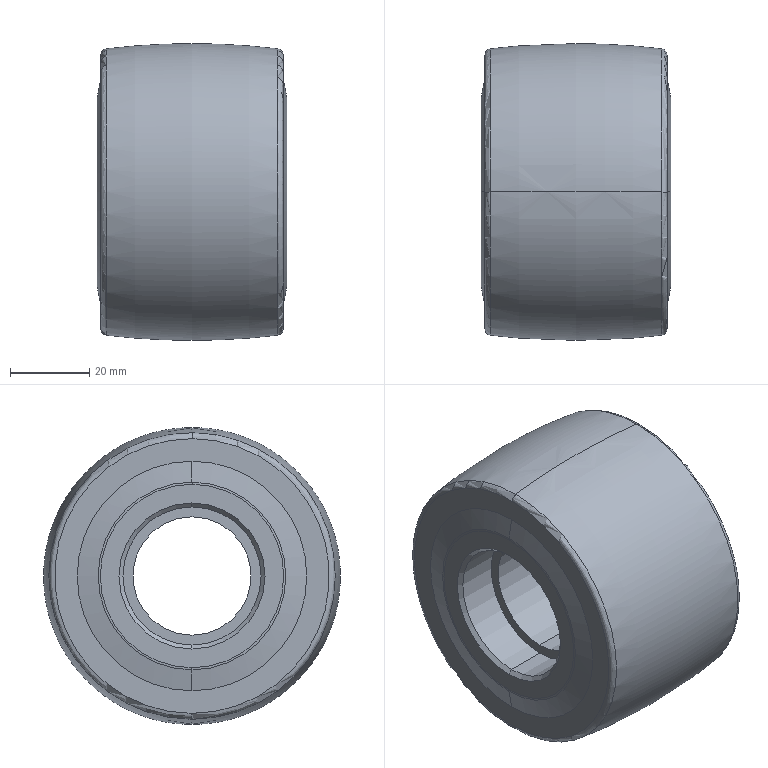Part | NX | features solid 2 | 1 solid | 30 faces | box 48 x 75 x 75 mm | volume 162673 mm3 | torus 10 | cone 8 | cylinder 6 | plane 6 | commonest cylinder face diameters 34.9 x4 29.9 x2
STEP:
#1=CARTESIAN_POINT('',(177.1,-71.5,-939.05));
#2=VERTEX_POINT('',#1);
#3=CARTESIAN_POINT('',(202.9,-71.5,-939.05));
#4=VERTEX_POINT('',#3);
#5=CARTESIAN_POINT('',(202.9,-71.5,-939.05));
#6=DIRECTION('',(-1.,0.,0.));
#7=VECTOR('',#6,1000.);
#8=LINE('',#5,#7);
#9=EDGE_CURVE('',#2,#4,#8,.F.);
#10=ORIENTED_EDGE('',*,*,#9,.T.);
#11=CARTESIAN_POINT('',(202.9,-71.5,-968.95));
#12=VERTEX_POINT('',#11);
#13=CARTESIAN_POINT('',(202.9,-71.5,-954.));
#14=DIRECTION('',(1.,0.,0.));
#15=DIRECTION('',(0.,0.,1.));
#16=AXIS2_PLACEMENT_3D('',#13,#14,#15);
#17=CIRCLE('',#16,14.95);
#18=EDGE_CURVE('',#4,#12,#17,.T.);
#19=ORIENTED_EDGE('',*,*,#18,.T.);
#20=CARTESIAN_POINT('',(177.1,-71.5,-968.95));
#21=VERTEX_POINT('',#20);
#22=CARTESIAN_POINT('',(202.9,-71.5,-968.95));
#23=DIRECTION('',(-1.,0.,0.));
#24=VECTOR('',#23,1000.);
#25=LINE('',#22,#24);
#26=EDGE_CURVE('',#12,#21,#25,.T.);
#27=ORIENTED_EDGE('',*,*,#26,.T.);
#28=CARTESIAN_POINT('',(177.1,-71.5,-954.));
#29=DIRECTION('',(-1.,0.,0.));
#30=DIRECTION('',(0.,0.,-1.));
#31=AXIS2_PLACEMENT_3D('',#28,#29,#30);
#32=CIRCLE('',#31,14.95);
#33=EDGE_CURVE('',#21,#2,#32,.T.);
#34=ORIENTED_EDGE('',*,*,#33,.T.);
#35=EDGE_LOOP('',(#10,#19,#27,#34));
#36=FACE_BOUND('',#35,.T.);
#37=CARTESIAN_POINT('',(163.6,-71.5,-954.));
#38=DIRECTION('',(1.,0.,0.));
#39=DIRECTION('',(0.,0.,1.));
#40=AXIS2_PLACEMENT_3D('',#37,#38,#39);
#41=CYLINDRICAL_SURFACE('',#40,14.95);
#42=ADVANCED_FACE('',(#36),#41,.F.);
#43=CARTESIAN_POINT('',(177.1,-71.5,-971.45));
#44=VERTEX_POINT('',#43);
#45=CARTESIAN_POINT('',(177.1,-71.5,-936.55));
#46=VERTEX_POINT('',#45);
#47=CARTESIAN_POINT('',(177.1,-71.5,-954.));
#48=DIRECTION('',(1.,0.,0.));
#49=DIRECTION('',(0.,0.,-1.));
#50=AXIS2_PLACEMENT_3D('',#47,#48,#49);
#51=CIRCLE('',#50,17.45);
#52=EDGE_CURVE('',#44,#46,#51,.T.);
#53=ORIENTED_EDGE('',*,*,#52,.F.);
#54=CARTESIAN_POINT('',(177.1,-71.5,-954.));
#55=DIRECTION('',(1.,0.,0.));
#56=DIRECTION('',(0.,0.,1.));
#57=AXIS2_PLACEMENT_3D('',#54,#55,#56);
#58=CIRCLE('',#57,17.45);
#59=EDGE_CURVE('',#46,#44,#58,.T.);
#60=ORIENTED_EDGE('',*,*,#59,.F.);
#61=EDGE_LOOP('',(#53,#60));
#62=FACE_BOUND('',#61,.T.);
#63=CARTESIAN_POINT('',(177.1,-71.5,-954.));
#64=DIRECTION('',(-1.,0.,0.));
#65=DIRECTION('',(0.,0.,1.));
#66=AXIS2_PLACEMENT_3D('',#63,#64,#65);
#67=CIRCLE('',#66,14.95);
#68=EDGE_CURVE('',#2,#21,#67,.T.);
#69=ORIENTED_EDGE('',*,*,#68,.F.);
#70=ORIENTED_EDGE('',*,*,#33,.F.);
#71=EDGE_LOOP('',(#69,#70));
#72=FACE_BOUND('',#71,.T.);
#73=CARTESIAN_POINT('',(177.1,-71.5,-954.));
#74=DIRECTION('',(1.,0.,0.));
#75=DIRECTION('',(0.,0.,1.));
#76=AXIS2_PLACEMENT_3D('',#73,#74,#75);
#77=PLANE('',#76);
#78=ADVANCED_FACE('',(#62,#72),#77,.F.);
#79=CARTESIAN_POINT('',(167.,-71.5,-936.55));
#80=VERTEX_POINT('',#79);
#81=CARTESIAN_POINT('',(177.1,-71.5,-936.55));
#82=DIRECTION('',(-1.,0.,0.));
#83=VECTOR('',#82,1000.);
#84=LINE('',#81,#83);
#85=EDGE_CURVE('',#80,#46,#84,.F.);
#86=ORIENTED_EDGE('',*,*,#85,.T.);
#87=ORIENTED_EDGE('',*,*,#59,.T.);
#88=CARTESIAN_POINT('',(167.,-71.5,-971.45));
#89=VERTEX_POINT('',#88);
#90=CARTESIAN_POINT('',(177.1,-71.5,-971.45));
#91=DIRECTION('',(-1.,0.,0.));
#92=VECTOR('',#91,1000.);
#93=LINE('',#90,#92);
#94=EDGE_CURVE('',#44,#89,#93,.T.);
#95=ORIENTED_EDGE('',*,*,#94,.T.);
#96=CARTESIAN_POINT('',(167.,-71.5,-954.));
#97=DIRECTION('',(-1.,0.,0.));
#98=DIRECTION('',(0.,0.,-1.));
#99=AXIS2_PLACEMENT_3D('',#96,#97,#98);
#100=CIRCLE('',#99,17.45);
#101=EDGE_CURVE('',#89,#80,#100,.T.);
#102=ORIENTED_EDGE('',*,*,#101,.T.);
#103=EDGE_LOOP('',(#86,#87,#95,#102));
#104=FACE_BOUND('',#103,.T.);
#105=CARTESIAN_POINT('',(163.6,-71.5,-954.));
#106=DIRECTION('',(1.,0.,0.));
#107=DIRECTION('',(0.,0.,1.));
#108=AXIS2_PLACEMENT_3D('',#105,#106,#107);
#109=CYLINDRICAL_SURFACE('',#108,17.45);
#110=ADVANCED_FACE('',(#104),#109,.F.);
#111=CARTESIAN_POINT('',(166.,-71.5,-972.45));
#112=VERTEX_POINT('',#111);
#113=CARTESIAN_POINT('',(166.,-71.5,-972.45));
#114=DIRECTION('',(0.7071,0.,0.7071));
#115=VECTOR('',#114,1000.);
#116=LINE('',#113,#115);
#117=EDGE_CURVE('',#112,#89,#116,.T.);
#118=ORIENTED_EDGE('',*,*,#117,.F.);
#119=CARTESIAN_POINT('',(166.,-71.5,-935.55));
#120=VERTEX_POINT('',#119);
#121=CARTESIAN_POINT('',(166.,-71.5,-954.));
#122=DIRECTION('',(-1.,0.,0.));
#123=DIRECTION('',(0.,0.,-1.));
#124=AXIS2_PLACEMENT_3D('',#121,#122,#123);
#125=CIRCLE('',#124,18.45);
#126=EDGE_CURVE('',#112,#120,#125,.T.);
#127=ORIENTED_EDGE('',*,*,#126,.T.);
#128=CARTESIAN_POINT('',(166.,-71.5,-935.55));
#129=DIRECTION('',(0.7071,0.,-0.7071));
#130=VECTOR('',#129,1000.);
#131=LINE('',#128,#130);
#132=EDGE_CURVE('',#80,#120,#131,.F.);
#133=ORIENTED_EDGE('',*,*,#132,.F.);
#134=ORIENTED_EDGE('',*,*,#101,.F.);
#135=EDGE_LOOP('',(#118,#127,#133,#134));
#136=FACE_BOUND('',#135,.T.);
#137=CARTESIAN_POINT('',(166.5,-71.5,-954.));
#138=DIRECTION('',(-1.,0.,0.));
#139=DIRECTION('',(0.,0.,-1.));
#140=AXIS2_PLACEMENT_3D('',#137,#138,#139);
#141=CONICAL_SURFACE('',#140,17.95,0.7854);
#142=ADVANCED_FACE('',(#136),#141,.F.);
#143=CARTESIAN_POINT('',(167.,-71.5,-954.));
#144=DIRECTION('',(-1.,0.,0.));
#145=DIRECTION('',(0.,0.,1.));
#146=AXIS2_PLACEMENT_3D('',#143,#144,#145);
#147=CIRCLE('',#146,17.45);
#148=EDGE_CURVE('',#80,#89,#147,.T.);
#149=ORIENTED_EDGE('',*,*,#148,.F.);
#150=ORIENTED_EDGE('',*,*,#132,.T.);
#151=CARTESIAN_POINT('',(166.,-71.5,-954.));
#152=DIRECTION('',(-1.,0.,0.));
#153=DIRECTION('',(0.,0.,1.));
#154=AXIS2_PLACEMENT_3D('',#151,#152,#153);
#155=CIRCLE('',#154,18.45);
#156=EDGE_CURVE('',#120,#112,#155,.T.);
#157=ORIENTED_EDGE('',*,*,#156,.T.);
#158=ORIENTED_EDGE('',*,*,#117,.T.);
#159=EDGE_LOOP('',(#149,#150,#157,#158));
#160=FACE_BOUND('',#159,.T.);
#161=CARTESIAN_POINT('',(166.5,-71.5,-954.));
#162=DIRECTION('',(-1.,0.,0.));
#163=DIRECTION('',(0.,0.,-1.));
#164=AXIS2_PLACEMENT_3D('',#161,#162,#163);
#165=CONICAL_SURFACE('',#164,17.95,0.7854);
#166=ADVANCED_FACE('',(#160),#165,.F.);
#167=CARTESIAN_POINT('',(166.,-71.724,-930.819));
#168=VERTEX_POINT('',#167);
#169=CARTESIAN_POINT('',(166.,-71.501,-977.182));
#170=VERTEX_POINT('',#169);
#171=CARTESIAN_POINT('',(166.,-71.5,-954.));
#172=DIRECTION('',(1.,0.,0.));
#173=DIRECTION('',(0.,-0.009654,1.));
#174=AXIS2_PLACEMENT_3D('',#171,#172,#173);
#175=CIRCLE('',#174,23.182);
#176=EDGE_CURVE('',#168,#170,#175,.T.);
#177=ORIENTED_EDGE('',*,*,#176,.F.);
#178=CARTESIAN_POINT('',(166.,-71.499,-930.818));
#179=VERTEX_POINT('',#178);
#180=CARTESIAN_POINT('',(166.,-71.5,-954.));
#181=DIRECTION('',(-1.,0.,0.));
#182=DIRECTION('',(0.,-0.009654,1.));
#183=AXIS2_PLACEMENT_3D('',#180,#181,#182);
#184=CIRCLE('',#183,23.182);
#185=EDGE_CURVE('',#168,#179,#184,.T.);
#186=ORIENTED_EDGE('',*,*,#185,.T.);
#187=CARTESIAN_POINT('',(166.,-71.276,-977.181));
#188=VERTEX_POINT('',#187);
#189=CARTESIAN_POINT('',(166.,-71.5,-954.));
#190=DIRECTION('',(1.,0.,0.));
#191=DIRECTION('',(0.,0.009654,-1.));
#192=AXIS2_PLACEMENT_3D('',#189,#190,#191);
#193=CIRCLE('',#192,23.182);
#194=EDGE_CURVE('',#179,#188,#193,.F.);
#195=ORIENTED_EDGE('',*,*,#194,.T.);
#196=CARTESIAN_POINT('',(166.,-71.5,-954.));
#197=DIRECTION('',(-1.,0.,0.));
#198=DIRECTION('',(0.,0.009654,-1.));
#199=AXIS2_PLACEMENT_3D('',#196,#197,#198);
#200=CIRCLE('',#199,23.182);
#201=EDGE_CURVE('',#170,#188,#200,.F.);
#202=ORIENTED_EDGE('',*,*,#201,.F.);
#203=EDGE_LOOP('',(#177,#186,#195,#202));
#204=FACE_BOUND('',#203,.T.);
#205=ORIENTED_EDGE('',*,*,#126,.F.);
#206=ORIENTED_EDGE('',*,*,#156,.F.);
#207=EDGE_LOOP('',(#205,#206));
#208=FACE_BOUND('',#207,.T.);
#209=CARTESIAN_POINT('',(166.,-71.5,-954.));
#210=DIRECTION('',(1.,0.,0.));
#211=DIRECTION('',(0.,0.,1.));
#212=AXIS2_PLACEMENT_3D('',#209,#210,#211);
#213=PLANE('',#212);
#214=ADVANCED_FACE('',(#204,#208),#213,.F.);
#215=CARTESIAN_POINT('',(166.048,-71.73,-930.287));
#216=VERTEX_POINT('',#215);
#217=CARTESIAN_POINT('',(169.,-71.725,-930.819));
#218=DIRECTION('',(0.,1.,0.009697));
#219=DIRECTION('',(-1.,0.000000003,-0.000000355));
#220=AXIS2_PLACEMENT_3D('',#217,#218,#219);
#221=CIRCLE('',#220,3.);
#222=EDGE_CURVE('',#168,#216,#221,.T.);
#223=ORIENTED_EDGE('',*,*,#222,.F.);
#224=ORIENTED_EDGE('',*,*,#176,.T.);
#225=ORIENTED_EDGE('',*,*,#201,.T.);
#226=CARTESIAN_POINT('',(166.048,-71.27,-977.713));
#227=VERTEX_POINT('',#226);
#228=CARTESIAN_POINT('',(169.,-71.275,-977.181));
#229=DIRECTION('',(0.,-1.,-0.009697));
#230=DIRECTION('',(-1.,-0.000000003,0.000000355));
#231=AXIS2_PLACEMENT_3D('',#228,#229,#230);
#232=CIRCLE('',#231,3.);
#233=EDGE_CURVE('',#227,#188,#232,.F.);
#234=ORIENTED_EDGE('',*,*,#233,.F.);
#235=CARTESIAN_POINT('',(166.048,-71.5,-977.714));
#236=VERTEX_POINT('',#235);
#237=CARTESIAN_POINT('',(166.048,-71.5,-954.));
#238=DIRECTION('',(1.,0.,0.));
#239=DIRECTION('',(0.,0.,-1.));
#240=AXIS2_PLACEMENT_3D('',#237,#238,#239);
#241=CIRCLE('',#240,23.714);
#242=EDGE_CURVE('',#236,#227,#241,.T.);
#243=ORIENTED_EDGE('',*,*,#242,.F.);
#244=CARTESIAN_POINT('',(166.048,-71.5,-954.));
#245=DIRECTION('',(1.,0.,0.));
#246=DIRECTION('',(0.,-0.009697,1.));
#247=AXIS2_PLACEMENT_3D('',#244,#245,#246);
#248=CIRCLE('',#247,23.714);
#249=EDGE_CURVE('',#216,#236,#248,.T.);
#250=ORIENTED_EDGE('',*,*,#249,.F.);
#251=EDGE_LOOP('',(#223,#224,#225,#234,#243,#250));
#252=FACE_BOUND('',#251,.T.);
#253=CARTESIAN_POINT('',(169.,-71.5,-954.));
#254=DIRECTION('',(-1.,0.,0.));
#255=DIRECTION('',(0.,0.009697,-1.));
#256=AXIS2_PLACEMENT_3D('',#253,#254,#255);
#257=TOROIDAL_SURFACE('',#256,23.182,3.);
#258=ADVANCED_FACE('',(#252),#257,.T.);
#259=CARTESIAN_POINT('',(166.048,-71.5,-930.286));
#260=VERTEX_POINT('',#259);
#261=CARTESIAN_POINT('',(166.048,-71.5,-954.));
#262=DIRECTION('',(1.,0.,0.));
#263=DIRECTION('',(0.,0.,1.));
#264=AXIS2_PLACEMENT_3D('',#261,#262,#263);
#265=CIRCLE('',#264,23.714);
#266=EDGE_CURVE('',#260,#216,#265,.T.);
#267=ORIENTED_EDGE('',*,*,#266,.T.);
#268=ORIENTED_EDGE('',*,*,#249,.T.);
#269=CARTESIAN_POINT('',(167.,-71.5,-983.));
#270=VERTEX_POINT('',#269);
#271=CARTESIAN_POINT('',(167.,-71.5,-983.));
#272=DIRECTION('',(-0.1773,0.,0.9842));
#273=VECTOR('',#272,1000.);
#274=LINE('',#271,#273);
#275=EDGE_CURVE('',#236,#270,#274,.F.);
#276=ORIENTED_EDGE('',*,*,#275,.T.);
#277=CARTESIAN_POINT('',(167.,-71.5,-925.));
#278=VERTEX_POINT('',#277);
#279=CARTESIAN_POINT('',(167.,-71.5,-954.));
#280=DIRECTION('',(-1.,0.,0.));
#281=DIRECTION('',(0.,0.,-1.));
#282=AXIS2_PLACEMENT_3D('',#279,#280,#281);
#283=CIRCLE('',#282,29.);
#284=EDGE_CURVE('',#270,#278,#283,.T.);
#285=ORIENTED_EDGE('',*,*,#284,.T.);
#286=CARTESIAN_POINT('',(167.,-71.5,-925.));
#287=DIRECTION('',(-0.1773,0.,-0.9842));
#288=VECTOR('',#287,1000.);
#289=LINE('',#286,#288);
#290=EDGE_CURVE('',#278,#260,#289,.T.);
#291=ORIENTED_EDGE('',*,*,#290,.T.);
#292=EDGE_LOOP('',(#267,#268,#276,#285,#291));
#293=FACE_BOUND('',#292,.T.);
#294=CARTESIAN_POINT('',(166.524,-71.5,-954.));
#295=DIRECTION('',(1.,0.,0.));
#296=DIRECTION('',(0.,0.,1.));
#297=AXIS2_PLACEMENT_3D('',#294,#295,#296);
#298=CONICAL_SURFACE('',#297,26.357,1.393);
#299=ADVANCED_FACE('',(#293),#298,.T.);
#300=CARTESIAN_POINT('',(166.048,-71.5,-954.));
#301=DIRECTION('',(1.,0.,0.));
#302=DIRECTION('',(0.,0.009697,-1.));
#303=AXIS2_PLACEMENT_3D('',#300,#301,#302);
#304=CIRCLE('',#303,23.714);
#305=EDGE_CURVE('',#227,#260,#304,.T.);
#306=ORIENTED_EDGE('',*,*,#305,.T.);
#307=ORIENTED_EDGE('',*,*,#290,.F.);
#308=CARTESIAN_POINT('',(167.,-71.5,-954.));
#309=DIRECTION('',(-1.,0.,0.));
#310=DIRECTION('',(0.,0.,1.));
#311=AXIS2_PLACEMENT_3D('',#308,#309,#310);
#312=CIRCLE('',#311,29.);
#313=EDGE_CURVE('',#278,#270,#312,.T.);
#314=ORIENTED_EDGE('',*,*,#313,.T.);
#315=ORIENTED_EDGE('',*,*,#275,.F.);
#316=ORIENTED_EDGE('',*,*,#242,.T.);
#317=EDGE_LOOP('',(#306,#307,#314,#315,#316));
#318=FACE_BOUND('',#317,.T.);
#319=CARTESIAN_POINT('',(166.524,-71.5,-954.));
#320=DIRECTION('',(1.,0.,0.));
#321=DIRECTION('',(0.,0.,1.));
#322=AXIS2_PLACEMENT_3D('',#319,#320,#321);
#323=CONICAL_SURFACE('',#322,26.357,1.393);
#324=ADVANCED_FACE('',(#318),#323,.T.);
#325=CARTESIAN_POINT('',(167.,-71.5,-988.7));
#326=VERTEX_POINT('',#325);
#327=CARTESIAN_POINT('',(167.,-71.735,-919.3));
#328=VERTEX_POINT('',#327);
#329=CARTESIAN_POINT('',(167.,-71.5,-954.));
#330=DIRECTION('',(1.,0.,0.));
#331=DIRECTION('',(0.,-0.006781,1.));
#332=AXIS2_PLACEMENT_3D('',#329,#330,#331);
#333=CIRCLE('',#332,34.7);
#334=EDGE_CURVE('',#326,#328,#333,.F.);
#335=ORIENTED_EDGE('',*,*,#334,.T.);
#336=CARTESIAN_POINT('',(167.,-71.5,-919.3));
#337=VERTEX_POINT('',#336);
#338=CARTESIAN_POINT('',(167.,-71.5,-954.));
#339=DIRECTION('',(-1.,0.,0.));
#340=DIRECTION('',(0.,-0.006781,1.));
#341=AXIS2_PLACEMENT_3D('',#338,#339,#340);
#342=CIRCLE('',#341,34.7);
#343=EDGE_CURVE('',#337,#328,#342,.F.);
#344=ORIENTED_EDGE('',*,*,#343,.F.);
#345=CARTESIAN_POINT('',(167.,-71.266,-988.7));
#346=VERTEX_POINT('',#345);
#347=CARTESIAN_POINT('',(167.,-71.5,-954.));
#348=DIRECTION('',(1.,0.,0.));
#349=DIRECTION('',(0.,0.006754,-1.));
#350=AXIS2_PLACEMENT_3D('',#347,#348,#349);
#351=CIRCLE('',#350,34.7);
#352=EDGE_CURVE('',#346,#337,#351,.T.);
#353=ORIENTED_EDGE('',*,*,#352,.F.);
#354=CARTESIAN_POINT('',(167.,-71.5,-954.));
#355=DIRECTION('',(-1.,0.,0.));
#356=DIRECTION('',(0.,0.006754,-1.));
#357=AXIS2_PLACEMENT_3D('',#354,#355,#356);
#358=CIRCLE('',#357,34.7);
#359=EDGE_CURVE('',#346,#326,#358,.T.);
#360=ORIENTED_EDGE('',*,*,#359,.T.);
#361=EDGE_LOOP('',(#335,#344,#353,#360));
#362=FACE_BOUND('',#361,.T.);
#363=ORIENTED_EDGE('',*,*,#313,.F.);
#364=ORIENTED_EDGE('',*,*,#284,.F.);
#365=EDGE_LOOP('',(#363,#364));
#366=FACE_BOUND('',#365,.T.);
#367=CARTESIAN_POINT('',(167.,-71.5,-954.));
#368=DIRECTION('',(1.,0.,0.));
#369=DIRECTION('',(0.,0.,1.));
#370=AXIS2_PLACEMENT_3D('',#367,#368,#369);
#371=PLANE('',#370);
#372=ADVANCED_FACE('',(#362,#366),#371,.F.);
#373=CARTESIAN_POINT('',(168.319,-71.745,-917.811));
#374=VERTEX_POINT('',#373);
#375=CARTESIAN_POINT('',(168.5,-71.735,-919.3));
#376=DIRECTION('',(0.,1.,0.00678));
#377=DIRECTION('',(-1.,0.000000842,-0.0001242));
#378=AXIS2_PLACEMENT_3D('',#375,#376,#377);
#379=CIRCLE('',#378,1.5);
#380=EDGE_CURVE('',#374,#328,#379,.F.);
#381=ORIENTED_EDGE('',*,*,#380,.T.);
#382=ORIENTED_EDGE('',*,*,#334,.F.);
#383=ORIENTED_EDGE('',*,*,#359,.F.);
#384=CARTESIAN_POINT('',(168.319,-71.255,-990.189));
#385=VERTEX_POINT('',#384);
#386=CARTESIAN_POINT('',(168.5,-71.265,-988.7));
#387=DIRECTION('',(0.,-1.,-0.006781));
#388=DIRECTION('',(-1.,-0.000000822,0.0001213));
#389=AXIS2_PLACEMENT_3D('',#386,#387,#388);
#390=CIRCLE('',#389,1.5);
#391=EDGE_CURVE('',#346,#385,#390,.T.);
#392=ORIENTED_EDGE('',*,*,#391,.T.);
#393=CARTESIAN_POINT('',(168.319,-71.5,-990.19));
#394=VERTEX_POINT('',#393);
#395=CARTESIAN_POINT('',(168.319,-71.5,-954.));
#396=DIRECTION('',(-1.,0.,0.));
#397=DIRECTION('',(0.,0.006782,-1.));
#398=AXIS2_PLACEMENT_3D('',#395,#396,#397);
#399=CIRCLE('',#398,36.19);
#400=EDGE_CURVE('',#385,#394,#399,.T.);
#401=ORIENTED_EDGE('',*,*,#400,.T.);
#402=CARTESIAN_POINT('',(168.319,-71.937,-990.187));
#403=VERTEX_POINT('',#402);
#404=CARTESIAN_POINT('',(168.319,-71.5,-954.));
#405=DIRECTION('',(-1.,0.,0.));
#406=DIRECTION('',(0.,-0.000002326,-1.));
#407=AXIS2_PLACEMENT_3D('',#404,#405,#406);
#408=CIRCLE('',#407,36.19);
#409=EDGE_CURVE('',#394,#403,#408,.T.);
#410=ORIENTED_EDGE('',*,*,#409,.T.);
#411=CARTESIAN_POINT('',(168.319,-71.5,-954.));
#412=DIRECTION('',(-1.,0.,0.));
#413=DIRECTION('',(0.,-0.01207,-0.9999));
#414=AXIS2_PLACEMENT_3D('',#411,#412,#413);
#415=CIRCLE('',#414,36.19);
#416=EDGE_CURVE('',#403,#374,#415,.T.);
#417=ORIENTED_EDGE('',*,*,#416,.T.);
#418=EDGE_LOOP('',(#381,#382,#383,#392,#401,#410,#417));
#419=FACE_BOUND('',#418,.T.);
#420=CARTESIAN_POINT('',(168.5,-71.5,-954.));
#421=DIRECTION('',(-1.,0.,0.));
#422=DIRECTION('',(0.,-0.01207,-0.9999));
#423=AXIS2_PLACEMENT_3D('',#420,#421,#422);
#424=TOROIDAL_SURFACE('',#423,34.7,1.5);
#425=ADVANCED_FACE('',(#419),#424,.T.);
#426=CARTESIAN_POINT('',(168.319,-71.5,-917.81));
#427=VERTEX_POINT('',#426);
#428=CARTESIAN_POINT('',(190.,-71.5,-916.5));
#429=VERTEX_POINT('',#428);
#430=CARTESIAN_POINT('',(190.,-71.5,-1096.5));
#431=DIRECTION('',(0.,-1.,0.));
#432=DIRECTION('',(0.,0.,1.));
#433=AXIS2_PLACEMENT_3D('',#430,#431,#432);
#434=CIRCLE('',#433,180.);
#435=EDGE_CURVE('',#427,#429,#434,.F.);
#436=ORIENTED_EDGE('',*,*,#435,.F.);
#437=CARTESIAN_POINT('',(168.319,-71.5,-954.));
#438=DIRECTION('',(-1.,0.,0.));
#439=DIRECTION('',(0.,-0.006783,1.));
#440=AXIS2_PLACEMENT_3D('',#437,#438,#439);
#441=CIRCLE('',#440,36.19);
#442=EDGE_CURVE('',#374,#427,#441,.T.);
#443=ORIENTED_EDGE('',*,*,#442,.F.);
#444=ORIENTED_EDGE('',*,*,#416,.F.);
#445=ORIENTED_EDGE('',*,*,#409,.F.);
#446=CARTESIAN_POINT('',(190.,-71.5,-991.5));
#447=VERTEX_POINT('',#446);
#448=CARTESIAN_POINT('',(190.,-71.5,-811.5));
#449=DIRECTION('',(0.,1.,0.));
#450=DIRECTION('',(0.,0.,-1.));
#451=AXIS2_PLACEMENT_3D('',#448,#449,#450);
#452=CIRCLE('',#451,180.);
#453=EDGE_CURVE('',#447,#394,#452,.T.);
#454=ORIENTED_EDGE('',*,*,#453,.F.);
#455=CARTESIAN_POINT('',(211.681,-71.5,-990.19));
#456=VERTEX_POINT('',#455);
#457=CARTESIAN_POINT('',(190.,-71.5,-811.5));
#458=DIRECTION('',(0.,1.,0.));
#459=DIRECTION('',(0.1204,0.,-0.9927));
#460=AXIS2_PLACEMENT_3D('',#457,#458,#459);
#461=CIRCLE('',#460,180.);
#462=EDGE_CURVE('',#456,#447,#461,.T.);
#463=ORIENTED_EDGE('',*,*,#462,.F.);
#464=CARTESIAN_POINT('',(211.681,-71.666,-917.811));
#465=VERTEX_POINT('',#464);
#466=CARTESIAN_POINT('',(211.681,-71.5,-954.));
#467=DIRECTION('',(1.,0.,0.));
#468=DIRECTION('',(0.,-0.004589,1.));
#469=AXIS2_PLACEMENT_3D('',#466,#467,#468);
#470=CIRCLE('',#469,36.19);
#471=EDGE_CURVE('',#465,#456,#470,.T.);
#472=ORIENTED_EDGE('',*,*,#471,.F.);
#473=CARTESIAN_POINT('',(211.681,-71.5,-917.81));
#474=VERTEX_POINT('',#473);
#475=CARTESIAN_POINT('',(211.681,-71.5,-954.));
#476=DIRECTION('',(1.,0.,0.));
#477=DIRECTION('',(0.,0.,1.));
#478=AXIS2_PLACEMENT_3D('',#475,#476,#477);
#479=CIRCLE('',#478,36.19);
#480=EDGE_CURVE('',#474,#465,#479,.T.);
#481=ORIENTED_EDGE('',*,*,#480,.F.);
#482=CARTESIAN_POINT('',(190.,-71.5,-1096.5));
#483=DIRECTION('',(0.,-1.,0.));
#484=DIRECTION('',(0.1204,0.,0.9927));
#485=AXIS2_PLACEMENT_3D('',#482,#483,#484);
#486=CIRCLE('',#485,180.);
#487=EDGE_CURVE('',#429,#474,#486,.F.);
#488=ORIENTED_EDGE('',*,*,#487,.F.);
#489=EDGE_LOOP('',(#436,#443,#444,#445,#454,#463,#472,#481,#488));
#490=FACE_BOUND('',#489,.T.);
#491=CARTESIAN_POINT('',(190.,-71.5,-954.));
#492=DIRECTION('',(1.,0.,0.));
#493=DIRECTION('',(0.,-1.,0.));
#494=AXIS2_PLACEMENT_3D('',#491,#492,#493);
#495=DEGENERATE_TOROIDAL_SURFACE('',#494,142.5,180.,.F.);
#496=ADVANCED_FACE('',(#490),#495,.F.);
#497=ORIENTED_EDGE('',*,*,#435,.T.);
#498=ORIENTED_EDGE('',*,*,#487,.T.);
#499=CARTESIAN_POINT('',(211.681,-71.334,-990.189));
#500=VERTEX_POINT('',#499);
#501=CARTESIAN_POINT('',(211.681,-71.5,-954.));
#502=DIRECTION('',(1.,0.,0.));
#503=DIRECTION('',(0.,0.00459,-1.));
#504=AXIS2_PLACEMENT_3D('',#501,#502,#503);
#505=CIRCLE('',#504,36.19);
#506=EDGE_CURVE('',#500,#474,#505,.T.);
#507=ORIENTED_EDGE('',*,*,#506,.F.);
#508=CARTESIAN_POINT('',(211.681,-71.5,-954.));
#509=DIRECTION('',(1.,0.,0.));
#510=DIRECTION('',(0.,0.,-1.));
#511=AXIS2_PLACEMENT_3D('',#508,#509,#510);
#512=CIRCLE('',#511,36.19);
#513=EDGE_CURVE('',#456,#500,#512,.T.);
#514=ORIENTED_EDGE('',*,*,#513,.F.);
#515=ORIENTED_EDGE('',*,*,#462,.T.);
#516=ORIENTED_EDGE('',*,*,#453,.T.);
#517=ORIENTED_EDGE('',*,*,#400,.F.);
#518=CARTESIAN_POINT('',(168.319,-71.5,-954.));
#519=DIRECTION('',(-1.,0.,0.));
#520=DIRECTION('',(0.,0.000002286,1.));
#521=AXIS2_PLACEMENT_3D('',#518,#519,#520);
#522=CIRCLE('',#521,36.19);
#523=EDGE_CURVE('',#427,#385,#522,.T.);
#524=ORIENTED_EDGE('',*,*,#523,.F.);
#525=EDGE_LOOP('',(#497,#498,#507,#514,#515,#516,#517,#524));
#526=FACE_BOUND('',#525,.T.);
#527=CARTESIAN_POINT('',(190.,-71.5,-954.));
#528=DIRECTION('',(1.,0.,0.));
#529=DIRECTION('',(0.,-1.,0.));
#530=AXIS2_PLACEMENT_3D('',#527,#528,#529);
#531=DEGENERATE_TOROIDAL_SURFACE('',#530,142.5,180.,.F.);
#532=ADVANCED_FACE('',(#526),#531,.F.);
#533=ORIENTED_EDGE('',*,*,#442,.T.);
#534=ORIENTED_EDGE('',*,*,#523,.T.);
#535=ORIENTED_EDGE('',*,*,#391,.F.);
#536=ORIENTED_EDGE('',*,*,#352,.T.);
#537=ORIENTED_EDGE('',*,*,#343,.T.);
#538=ORIENTED_EDGE('',*,*,#380,.F.);
#539=EDGE_LOOP('',(#533,#534,#535,#536,#537,#538));
#540=FACE_BOUND('',#539,.T.);
#541=CARTESIAN_POINT('',(168.5,-71.5,-954.));
#542=DIRECTION('',(-1.,0.,0.));
#543=DIRECTION('',(0.,-0.006781,1.));
#544=AXIS2_PLACEMENT_3D('',#541,#542,#543);
#545=TOROIDAL_SURFACE('',#544,34.7,1.5);
#546=ADVANCED_FACE('',(#540),#545,.T.);
#547=CARTESIAN_POINT('',(213.,-71.659,-919.3));
#548=VERTEX_POINT('',#547);
#549=CARTESIAN_POINT('',(211.5,-71.659,-919.3));
#550=DIRECTION('',(0.,1.,0.00459));
#551=DIRECTION('',(0.1205,-0.004557,0.9927));
#552=AXIS2_PLACEMENT_3D('',#549,#550,#551);
#553=CIRCLE('',#552,1.5);
#554=EDGE_CURVE('',#465,#548,#553,.T.);
#555=ORIENTED_EDGE('',*,*,#554,.F.);
#556=ORIENTED_EDGE('',*,*,#471,.T.);
#557=ORIENTED_EDGE('',*,*,#513,.T.);
#558=CARTESIAN_POINT('',(213.,-71.341,-988.7));
#559=VERTEX_POINT('',#558);
#560=CARTESIAN_POINT('',(211.5,-71.341,-988.7));
#561=DIRECTION('',(0.,-1.,-0.00459));
#562=DIRECTION('',(0.1205,0.004557,-0.9927));
#563=AXIS2_PLACEMENT_3D('',#560,#561,#562);
#564=CIRCLE('',#563,1.5);
#565=EDGE_CURVE('',#559,#500,#564,.F.);
#566=ORIENTED_EDGE('',*,*,#565,.F.);
#567=CARTESIAN_POINT('',(213.,-71.5,-988.7));
#568=VERTEX_POINT('',#567);
#569=CARTESIAN_POINT('',(213.,-71.5,-954.));
#570=DIRECTION('',(1.,0.,0.));
#571=DIRECTION('',(0.,0.,-1.));
#572=AXIS2_PLACEMENT_3D('',#569,#570,#571);
#573=CIRCLE('',#572,34.7);
#574=EDGE_CURVE('',#559,#568,#573,.F.);
#575=ORIENTED_EDGE('',*,*,#574,.T.);
#576=CARTESIAN_POINT('',(213.,-71.5,-954.));
#577=DIRECTION('',(-1.,0.,0.));
#578=DIRECTION('',(0.,0.,-1.));
#579=AXIS2_PLACEMENT_3D('',#576,#577,#578);
#580=CIRCLE('',#579,34.7);
#581=EDGE_CURVE('',#568,#548,#580,.T.);
#582=ORIENTED_EDGE('',*,*,#581,.T.);
#583=EDGE_LOOP('',(#555,#556,#557,#566,#575,#582));
#584=FACE_BOUND('',#583,.T.);
#585=CARTESIAN_POINT('',(211.5,-71.5,-954.));
#586=DIRECTION('',(-1.,0.,0.));
#587=DIRECTION('',(0.,0.00459,-1.));
#588=AXIS2_PLACEMENT_3D('',#585,#586,#587);
#589=TOROIDAL_SURFACE('',#588,34.7,1.5);
#590=ADVANCED_FACE('',(#584),#589,.T.);
#591=CARTESIAN_POINT('',(213.,-71.5,-919.3));
#592=VERTEX_POINT('',#591);
#593=CARTESIAN_POINT('',(213.,-71.5,-954.));
#594=DIRECTION('',(1.,0.,0.));
#595=DIRECTION('',(0.,0.,1.));
#596=AXIS2_PLACEMENT_3D('',#593,#594,#595);
#597=CIRCLE('',#596,34.7);
#598=EDGE_CURVE('',#548,#592,#597,.F.);
#599=ORIENTED_EDGE('',*,*,#598,.F.);
#600=ORIENTED_EDGE('',*,*,#581,.F.);
#601=ORIENTED_EDGE('',*,*,#574,.F.);
#602=CARTESIAN_POINT('',(213.,-71.5,-954.));
#603=DIRECTION('',(-1.,0.,0.));
#604=DIRECTION('',(0.,0.,1.));
#605=AXIS2_PLACEMENT_3D('',#602,#603,#604);
#606=CIRCLE('',#605,34.7);
#607=EDGE_CURVE('',#592,#559,#606,.T.);
#608=ORIENTED_EDGE('',*,*,#607,.F.);
#609=EDGE_LOOP('',(#599,#600,#601,#608));
#610=FACE_BOUND('',#609,.T.);
#611=CARTESIAN_POINT('',(213.,-71.5,-925.));
#612=VERTEX_POINT('',#611);
#613=CARTESIAN_POINT('',(213.,-71.5,-983.));
#614=VERTEX_POINT('',#613);
#615=CARTESIAN_POINT('',(213.,-71.5,-954.));
#616=DIRECTION('',(1.,0.,0.));
#617=DIRECTION('',(0.,0.,1.));
#618=AXIS2_PLACEMENT_3D('',#615,#616,#617);
#619=CIRCLE('',#618,29.);
#620=EDGE_CURVE('',#612,#614,#619,.T.);
#621=ORIENTED_EDGE('',*,*,#620,.F.);
#622=CARTESIAN_POINT('',(213.,-71.5,-954.));
#623=DIRECTION('',(1.,0.,0.));
#624=DIRECTION('',(0.,0.,-1.));
#625=AXIS2_PLACEMENT_3D('',#622,#623,#624);
#626=CIRCLE('',#625,29.);
#627=EDGE_CURVE('',#614,#612,#626,.T.);
#628=ORIENTED_EDGE('',*,*,#627,.F.);
#629=EDGE_LOOP('',(#621,#628));
#630=FACE_BOUND('',#629,.T.);
#631=CARTESIAN_POINT('',(213.,-71.5,-954.));
#632=DIRECTION('',(1.,0.,0.));
#633=DIRECTION('',(0.,0.,1.));
#634=AXIS2_PLACEMENT_3D('',#631,#632,#633);
#635=PLANE('',#634);
#636=ADVANCED_FACE('',(#610,#630),#635,.T.);
#637=ORIENTED_EDGE('',*,*,#598,.T.);
#638=ORIENTED_EDGE('',*,*,#607,.T.);
#639=ORIENTED_EDGE('',*,*,#565,.T.);
#640=ORIENTED_EDGE('',*,*,#506,.T.);
#641=ORIENTED_EDGE('',*,*,#480,.T.);
#642=ORIENTED_EDGE('',*,*,#554,.T.);
#643=EDGE_LOOP('',(#637,#638,#639,#640,#641,#642));
#644=FACE_BOUND('',#643,.T.);
#645=CARTESIAN_POINT('',(211.5,-71.5,-954.));
#646=DIRECTION('',(-1.,0.,0.));
#647=DIRECTION('',(0.,-0.00459,1.));
#648=AXIS2_PLACEMENT_3D('',#645,#646,#647);
#649=TOROIDAL_SURFACE('',#648,34.7,1.5);
#650=ADVANCED_FACE('',(#644),#649,.T.);
#651=CARTESIAN_POINT('',(213.952,-71.344,-977.713));
#652=VERTEX_POINT('',#651);
#653=CARTESIAN_POINT('',(213.952,-71.5,-977.714));
#654=VERTEX_POINT('',#653);
#655=CARTESIAN_POINT('',(213.952,-71.5,-954.));
#656=DIRECTION('',(-1.,0.,0.));
#657=DIRECTION('',(0.,0.006563,-1.));
#658=AXIS2_PLACEMENT_3D('',#655,#656,#657);
#659=CIRCLE('',#658,23.714);
#660=EDGE_CURVE('',#652,#654,#659,.T.);
#661=ORIENTED_EDGE('',*,*,#660,.T.);
#662=CARTESIAN_POINT('',(213.,-71.5,-983.));
#663=DIRECTION('',(0.1773,0.,0.9842));
#664=VECTOR('',#663,1000.);
#665=LINE('',#662,#664);
#666=EDGE_CURVE('',#654,#614,#665,.F.);
#667=ORIENTED_EDGE('',*,*,#666,.T.);
#668=ORIENTED_EDGE('',*,*,#627,.T.);
#669=CARTESIAN_POINT('',(213.952,-71.5,-930.286));
#670=VERTEX_POINT('',#669);
#671=CARTESIAN_POINT('',(213.,-71.5,-925.));
#672=DIRECTION('',(0.1773,0.,-0.9842));
#673=VECTOR('',#672,1000.);
#674=LINE('',#671,#673);
#675=EDGE_CURVE('',#612,#670,#674,.T.);
#676=ORIENTED_EDGE('',*,*,#675,.T.);
#677=CARTESIAN_POINT('',(213.952,-71.5,-954.));
#678=DIRECTION('',(-1.,0.,0.));
#679=DIRECTION('',(0.,0.,1.));
#680=AXIS2_PLACEMENT_3D('',#677,#678,#679);
#681=CIRCLE('',#680,23.714);
#682=EDGE_CURVE('',#670,#652,#681,.T.);
#683=ORIENTED_EDGE('',*,*,#682,.T.);
#684=EDGE_LOOP('',(#661,#667,#668,#676,#683));
#685=FACE_BOUND('',#684,.T.);
#686=CARTESIAN_POINT('',(213.476,-71.5,-954.));
#687=DIRECTION('',(-1.,0.,0.));
#688=DIRECTION('',(0.,0.,-1.));
#689=AXIS2_PLACEMENT_3D('',#686,#687,#688);
#690=CONICAL_SURFACE('',#689,26.357,1.393);
#691=ADVANCED_FACE('',(#685),#690,.T.);
#692=CARTESIAN_POINT('',(214.,-71.5,-930.818));
#693=VERTEX_POINT('',#692);
#694=CARTESIAN_POINT('',(214.,-71.652,-930.819));
#695=VERTEX_POINT('',#694);
#696=CARTESIAN_POINT('',(214.,-71.5,-954.));
#697=DIRECTION('',(1.,0.,0.));
#698=DIRECTION('',(0.,-0.000000084,1.));
#699=AXIS2_PLACEMENT_3D('',#696,#697,#698);
#700=CIRCLE('',#699,23.182);
#701=EDGE_CURVE('',#693,#695,#700,.T.);
#702=ORIENTED_EDGE('',*,*,#701,.F.);
#703=CARTESIAN_POINT('',(214.,-71.348,-977.181));
#704=VERTEX_POINT('',#703);
#705=CARTESIAN_POINT('',(214.,-71.5,-954.));
#706=DIRECTION('',(-1.,0.,0.));
#707=DIRECTION('',(0.,-0.000000084,1.));
#708=AXIS2_PLACEMENT_3D('',#705,#706,#707);
#709=CIRCLE('',#708,23.182);
#710=EDGE_CURVE('',#704,#693,#709,.F.);
#711=ORIENTED_EDGE('',*,*,#710,.F.);
#712=CARTESIAN_POINT('',(211.,-71.348,-977.181));
#713=DIRECTION('',(0.,-1.,-0.006563));
#714=DIRECTION('',(0.9842,0.001164,-0.1773));
#715=AXIS2_PLACEMENT_3D('',#712,#713,#714);
#716=CIRCLE('',#715,3.);
#717=EDGE_CURVE('',#652,#704,#716,.T.);
#718=ORIENTED_EDGE('',*,*,#717,.F.);
#719=ORIENTED_EDGE('',*,*,#682,.F.);
#720=CARTESIAN_POINT('',(213.952,-71.656,-930.287));
#721=VERTEX_POINT('',#720);
#722=CARTESIAN_POINT('',(213.952,-71.5,-954.));
#723=DIRECTION('',(-1.,0.,0.));
#724=DIRECTION('',(0.,-0.006563,1.));
#725=AXIS2_PLACEMENT_3D('',#722,#723,#724);
#726=CIRCLE('',#725,23.714);
#727=EDGE_CURVE('',#721,#670,#726,.T.);
#728=ORIENTED_EDGE('',*,*,#727,.F.);
#729=CARTESIAN_POINT('',(211.,-71.652,-930.819));
#730=DIRECTION('',(0.,1.,0.006563));
#731=DIRECTION('',(0.9842,-0.001164,0.1773));
#732=AXIS2_PLACEMENT_3D('',#729,#730,#731);
#733=CIRCLE('',#732,3.);
#734=EDGE_CURVE('',#695,#721,#733,.F.);
#735=ORIENTED_EDGE('',*,*,#734,.F.);
#736=EDGE_LOOP('',(#702,#711,#718,#719,#728,#735));
#737=FACE_BOUND('',#736,.T.);
#738=CARTESIAN_POINT('',(211.,-71.5,-954.));
#739=DIRECTION('',(-1.,0.,0.));
#740=DIRECTION('',(0.,-0.006563,1.));
#741=AXIS2_PLACEMENT_3D('',#738,#739,#740);
#742=TOROIDAL_SURFACE('',#741,23.182,3.);
#743=ADVANCED_FACE('',(#737),#742,.T.);
#744=ORIENTED_EDGE('',*,*,#734,.T.);
#745=CARTESIAN_POINT('',(213.952,-71.5,-954.));
#746=DIRECTION('',(-1.,0.,0.));
#747=DIRECTION('',(0.,0.,-1.));
#748=AXIS2_PLACEMENT_3D('',#745,#746,#747);
#749=CIRCLE('',#748,23.714);
#750=EDGE_CURVE('',#654,#721,#749,.T.);
#751=ORIENTED_EDGE('',*,*,#750,.F.);
#752=ORIENTED_EDGE('',*,*,#660,.F.);
#753=ORIENTED_EDGE('',*,*,#717,.T.);
#754=CARTESIAN_POINT('',(214.,-71.5,-977.182));
#755=VERTEX_POINT('',#754);
#756=CARTESIAN_POINT('',(214.,-71.5,-954.));
#757=DIRECTION('',(1.,0.,0.));
#758=DIRECTION('',(0.,0.000000084,-1.));
#759=AXIS2_PLACEMENT_3D('',#756,#757,#758);
#760=CIRCLE('',#759,23.182);
#761=EDGE_CURVE('',#755,#704,#760,.T.);
#762=ORIENTED_EDGE('',*,*,#761,.F.);
#763=CARTESIAN_POINT('',(214.,-71.5,-954.));
#764=DIRECTION('',(-1.,0.,0.));
#765=DIRECTION('',(0.,0.000000084,-1.));
#766=AXIS2_PLACEMENT_3D('',#763,#764,#765);
#767=CIRCLE('',#766,23.182);
#768=EDGE_CURVE('',#695,#755,#767,.F.);
#769=ORIENTED_EDGE('',*,*,#768,.F.);
#770=EDGE_LOOP('',(#744,#751,#752,#753,#762,#769));
#771=FACE_BOUND('',#770,.T.);
#772=CARTESIAN_POINT('',(211.,-71.5,-954.));
#773=DIRECTION('',(-1.,0.,0.));
#774=DIRECTION('',(0.,0.006563,-1.));
#775=AXIS2_PLACEMENT_3D('',#772,#773,#774);
#776=TOROIDAL_SURFACE('',#775,23.182,3.);
#777=ADVANCED_FACE('',(#771),#776,.T.);
#778=ORIENTED_EDGE('',*,*,#701,.T.);
#779=ORIENTED_EDGE('',*,*,#768,.T.);
#780=ORIENTED_EDGE('',*,*,#761,.T.);
#781=ORIENTED_EDGE('',*,*,#710,.T.);
#782=EDGE_LOOP('',(#778,#779,#780,#781));
#783=FACE_BOUND('',#782,.T.);
#784=CARTESIAN_POINT('',(214.,-71.5,-972.45));
#785=VERTEX_POINT('',#784);
#786=CARTESIAN_POINT('',(214.,-71.5,-935.55));
#787=VERTEX_POINT('',#786);
#788=CARTESIAN_POINT('',(214.,-71.5,-954.));
#789=DIRECTION('',(1.,0.,0.));
#790=DIRECTION('',(0.,0.,-1.));
#791=AXIS2_PLACEMENT_3D('',#788,#789,#790);
#792=CIRCLE('',#791,18.45);
#793=EDGE_CURVE('',#785,#787,#792,.T.);
#794=ORIENTED_EDGE('',*,*,#793,.F.);
#795=CARTESIAN_POINT('',(214.,-71.5,-954.));
#796=DIRECTION('',(1.,0.,0.));
#797=DIRECTION('',(0.,0.,1.));
#798=AXIS2_PLACEMENT_3D('',#795,#796,#797);
#799=CIRCLE('',#798,18.45);
#800=EDGE_CURVE('',#787,#785,#799,.T.);
#801=ORIENTED_EDGE('',*,*,#800,.F.);
#802=EDGE_LOOP('',(#794,#801));
#803=FACE_BOUND('',#802,.T.);
#804=CARTESIAN_POINT('',(214.,-71.5,-954.));
#805=DIRECTION('',(1.,0.,0.));
#806=DIRECTION('',(0.,0.,1.));
#807=AXIS2_PLACEMENT_3D('',#804,#805,#806);
#808=PLANE('',#807);
#809=ADVANCED_FACE('',(#783,#803),#808,.T.);
#810=CARTESIAN_POINT('',(213.,-71.5,-936.55));
#811=VERTEX_POINT('',#810);
#812=CARTESIAN_POINT('',(214.,-71.5,-935.55));
#813=DIRECTION('',(-0.7071,0.,-0.7071));
#814=VECTOR('',#813,1000.);
#815=LINE('',#812,#814);
#816=EDGE_CURVE('',#787,#811,#815,.T.);
#817=ORIENTED_EDGE('',*,*,#816,.F.);
#818=ORIENTED_EDGE('',*,*,#800,.T.);
#819=CARTESIAN_POINT('',(213.,-71.5,-971.45));
#820=VERTEX_POINT('',#819);
#821=CARTESIAN_POINT('',(214.,-71.5,-972.45));
#822=DIRECTION('',(-0.7071,0.,0.7071));
#823=VECTOR('',#822,1000.);
#824=LINE('',#821,#823);
#825=EDGE_CURVE('',#820,#785,#824,.F.);
#826=ORIENTED_EDGE('',*,*,#825,.F.);
#827=CARTESIAN_POINT('',(213.,-71.5,-954.));
#828=DIRECTION('',(1.,0.,0.));
#829=DIRECTION('',(0.,0.,1.));
#830=AXIS2_PLACEMENT_3D('',#827,#828,#829);
#831=CIRCLE('',#830,17.45);
#832=EDGE_CURVE('',#811,#820,#831,.T.);
#833=ORIENTED_EDGE('',*,*,#832,.F.);
#834=EDGE_LOOP('',(#817,#818,#826,#833));
#835=FACE_BOUND('',#834,.T.);
#836=CARTESIAN_POINT('',(213.5,-71.5,-954.));
#837=DIRECTION('',(1.,0.,0.));
#838=DIRECTION('',(0.,0.,1.));
#839=AXIS2_PLACEMENT_3D('',#836,#837,#838);
#840=CONICAL_SURFACE('',#839,17.95,0.7854);
#841=ADVANCED_FACE('',(#835),#840,.F.);
#842=CARTESIAN_POINT('',(202.9,-71.5,-936.55));
#843=VERTEX_POINT('',#842);
#844=CARTESIAN_POINT('',(213.,-71.5,-936.55));
#845=DIRECTION('',(-1.,0.,0.));
#846=VECTOR('',#845,1000.);
#847=LINE('',#844,#846);
#848=EDGE_CURVE('',#811,#843,#847,.T.);
#849=ORIENTED_EDGE('',*,*,#848,.F.);
#850=ORIENTED_EDGE('',*,*,#832,.T.);
#851=CARTESIAN_POINT('',(202.9,-71.5,-971.45));
#852=VERTEX_POINT('',#851);
#853=CARTESIAN_POINT('',(213.,-71.5,-971.45));
#854=DIRECTION('',(-1.,0.,0.));
#855=VECTOR('',#854,1000.);
#856=LINE('',#853,#855);
#857=EDGE_CURVE('',#852,#820,#856,.F.);
#858=ORIENTED_EDGE('',*,*,#857,.F.);
#859=CARTESIAN_POINT('',(202.9,-71.5,-954.));
#860=DIRECTION('',(-1.,0.,0.));
#861=DIRECTION('',(0.,0.,-1.));
#862=AXIS2_PLACEMENT_3D('',#859,#860,#861);
#863=CIRCLE('',#862,17.45);
#864=EDGE_CURVE('',#852,#843,#863,.T.);
#865=ORIENTED_EDGE('',*,*,#864,.T.);
#866=EDGE_LOOP('',(#849,#850,#858,#865));
#867=FACE_BOUND('',#866,.T.);
#868=CARTESIAN_POINT('',(163.6,-71.5,-954.));
#869=DIRECTION('',(1.,0.,0.));
#870=DIRECTION('',(0.,0.,1.));
#871=AXIS2_PLACEMENT_3D('',#868,#869,#870);
#872=CYLINDRICAL_SURFACE('',#871,17.45);
#873=ADVANCED_FACE('',(#867),#872,.F.);
#874=ORIENTED_EDGE('',*,*,#864,.F.);
#875=CARTESIAN_POINT('',(202.9,-71.5,-954.));
#876=DIRECTION('',(-1.,0.,0.));
#877=DIRECTION('',(0.,0.,1.));
#878=AXIS2_PLACEMENT_3D('',#875,#876,#877);
#879=CIRCLE('',#878,17.45);
#880=EDGE_CURVE('',#843,#852,#879,.T.);
#881=ORIENTED_EDGE('',*,*,#880,.F.);
#882=EDGE_LOOP('',(#874,#881));
#883=FACE_BOUND('',#882,.T.);
#884=CARTESIAN_POINT('',(202.9,-71.5,-954.));
#885=DIRECTION('',(1.,0.,0.));
#886=DIRECTION('',(0.,0.,-1.));
#887=AXIS2_PLACEMENT_3D('',#884,#885,#886);
#888=CIRCLE('',#887,14.95);
#889=EDGE_CURVE('',#12,#4,#888,.T.);
#890=ORIENTED_EDGE('',*,*,#889,.F.);
#891=ORIENTED_EDGE('',*,*,#18,.F.);
#892=EDGE_LOOP('',(#890,#891));
#893=FACE_BOUND('',#892,.T.);
#894=CARTESIAN_POINT('',(202.9,-71.5,-954.));
#895=DIRECTION('',(1.,0.,0.));
#896=DIRECTION('',(0.,0.,1.));
#897=AXIS2_PLACEMENT_3D('',#894,#895,#896);
#898=PLANE('',#897);
#899=ADVANCED_FACE('',(#883,#893),#898,.T.);
#900=ORIENTED_EDGE('',*,*,#880,.T.);
#901=ORIENTED_EDGE('',*,*,#857,.T.);
#902=CARTESIAN_POINT('',(213.,-71.5,-954.));
#903=DIRECTION('',(1.,0.,0.));
#904=DIRECTION('',(0.,0.,-1.));
#905=AXIS2_PLACEMENT_3D('',#902,#903,#904);
#906=CIRCLE('',#905,17.45);
#907=EDGE_CURVE('',#820,#811,#906,.T.);
#908=ORIENTED_EDGE('',*,*,#907,.T.);
#909=ORIENTED_EDGE('',*,*,#848,.T.);
#910=EDGE_LOOP('',(#900,#901,#908,#909));
#911=FACE_BOUND('',#910,.T.);
#912=CARTESIAN_POINT('',(163.6,-71.5,-954.));
#913=DIRECTION('',(1.,0.,0.));
#914=DIRECTION('',(0.,0.,1.));
#915=AXIS2_PLACEMENT_3D('',#912,#913,#914);
#916=CYLINDRICAL_SURFACE('',#915,17.45);
#917=ADVANCED_FACE('',(#911),#916,.F.);
#918=ORIENTED_EDGE('',*,*,#907,.F.);
#919=ORIENTED_EDGE('',*,*,#825,.T.);
#920=ORIENTED_EDGE('',*,*,#793,.T.);
#921=ORIENTED_EDGE('',*,*,#816,.T.);
#922=EDGE_LOOP('',(#918,#919,#920,#921));
#923=FACE_BOUND('',#922,.T.);
#924=CARTESIAN_POINT('',(213.5,-71.5,-954.));
#925=DIRECTION('',(1.,0.,0.));
#926=DIRECTION('',(0.,0.,1.));
#927=AXIS2_PLACEMENT_3D('',#924,#925,#926);
#928=CONICAL_SURFACE('',#927,17.95,0.7854);
#929=ADVANCED_FACE('',(#923),#928,.F.);
#930=ORIENTED_EDGE('',*,*,#68,.T.);
#931=ORIENTED_EDGE('',*,*,#26,.F.);
#932=ORIENTED_EDGE('',*,*,#889,.T.);
#933=ORIENTED_EDGE('',*,*,#9,.F.);
#934=EDGE_LOOP('',(#930,#931,#932,#933));
#935=FACE_BOUND('',#934,.T.);
#936=CARTESIAN_POINT('',(163.6,-71.5,-954.));
#937=DIRECTION('',(1.,0.,0.));
#938=DIRECTION('',(0.,0.,1.));
#939=AXIS2_PLACEMENT_3D('',#936,#937,#938);
#940=CYLINDRICAL_SURFACE('',#939,14.95);
#941=ADVANCED_FACE('',(#935),#940,.F.);
#942=ORIENTED_EDGE('',*,*,#750,.T.);
#943=ORIENTED_EDGE('',*,*,#727,.T.);
#944=ORIENTED_EDGE('',*,*,#675,.F.);
#945=ORIENTED_EDGE('',*,*,#620,.T.);
#946=ORIENTED_EDGE('',*,*,#666,.F.);
#947=EDGE_LOOP('',(#942,#943,#944,#945,#946));
#948=FACE_BOUND('',#947,.T.);
#949=CARTESIAN_POINT('',(213.476,-71.5,-954.));
#950=DIRECTION('',(-1.,0.,0.));
#951=DIRECTION('',(0.,0.,-1.));
#952=AXIS2_PLACEMENT_3D('',#949,#950,#951);
#953=CONICAL_SURFACE('',#952,26.357,1.393);
#954=ADVANCED_FACE('',(#948),#953,.T.);
#955=ORIENTED_EDGE('',*,*,#266,.F.);
#956=ORIENTED_EDGE('',*,*,#305,.F.);
#957=ORIENTED_EDGE('',*,*,#233,.T.);
#958=ORIENTED_EDGE('',*,*,#194,.F.);
#959=ORIENTED_EDGE('',*,*,#185,.F.);
#960=ORIENTED_EDGE('',*,*,#222,.T.);
#961=EDGE_LOOP('',(#955,#956,#957,#958,#959,#960));
#962=FACE_BOUND('',#961,.T.);
#963=CARTESIAN_POINT('',(169.,-71.5,-954.));
#964=DIRECTION('',(-1.,0.,0.));
#965=DIRECTION('',(0.,-0.009697,1.));
#966=AXIS2_PLACEMENT_3D('',#963,#964,#965);
#967=TOROIDAL_SURFACE('',#966,23.182,3.);
#968=ADVANCED_FACE('',(#962),#967,.T.);
#969=ORIENTED_EDGE('',*,*,#148,.T.);
#970=ORIENTED_EDGE('',*,*,#94,.F.);
#971=ORIENTED_EDGE('',*,*,#52,.T.);
#972=ORIENTED_EDGE('',*,*,#85,.F.);
#973=EDGE_LOOP('',(#969,#970,#971,#972));
#974=FACE_BOUND('',#973,.T.);
#975=CARTESIAN_POINT('',(163.6,-71.5,-954.));
#976=DIRECTION('',(1.,0.,0.));
#977=DIRECTION('',(0.,0.,1.));
#978=AXIS2_PLACEMENT_3D('',#975,#976,#977);
#979=CYLINDRICAL_SURFACE('',#978,17.45);
#980=ADVANCED_FACE('',(#974),#979,.F.);
#981=CLOSED_SHELL('',(#42,#78,#110,#142,#166,#214,#258,#299,#324,#372,#425,#496,#532,#546,#590,#636,#650,#691,#743,#777,#809,#841,#873,#899,#917,#929,#941,#954,#968,#980));
#982=MANIFOLD_SOLID_BREP('',#981);
#983=(LENGTH_UNIT()NAMED_UNIT(*)SI_UNIT(.MILLI.,.METRE.));
#984=UNCERTAINTY_MEASURE_WITH_UNIT(LENGTH_MEASURE(0.00001),#983,'','');
#985=(NAMED_UNIT(*)PLANE_ANGLE_UNIT()SI_UNIT($,.RADIAN.));
#986=(NAMED_UNIT(*)SI_UNIT($,.STERADIAN.)SOLID_ANGLE_UNIT());
#987=(GEOMETRIC_REPRESENTATION_CONTEXT(3)GLOBAL_UNCERTAINTY_ASSIGNED_CONTEXT((#984))GLOBAL_UNIT_ASSIGNED_CONTEXT((#983,#985,#986))REPRESENTATION_CONTEXT('',''));
#988=ADVANCED_BREP_SHAPE_REPRESENTATION('',(#982),#987);